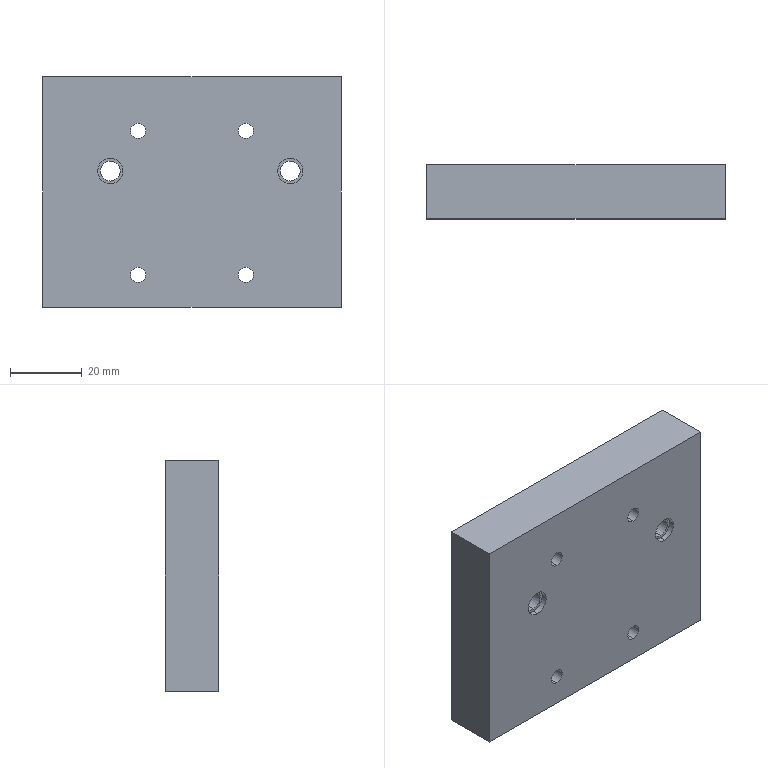Part | SolidWorks | features HoleWzd 2, ICE 2, Extrusion 1 | 1 solid | 36 faces | box 83 x 15 x 64 mm | volume 77222 mm3 | cylinder 24 | plane 12 | commonest cylinder face diameters 4.2 x8 5.5 x4 7 x4 9 x4 10 x4
STEP:
#1=CARTESIAN_POINT('',(56.5,12.9,44.5));
#2=VERTEX_POINT('',#1);
#3=CARTESIAN_POINT('',(56.5,12.9,53.5));
#4=VERTEX_POINT('',#3);
#5=CARTESIAN_POINT('',(56.5,12.9,49.));
#6=DIRECTION('',(0.,1.,0.));
#7=DIRECTION('',(0.,0.,1.));
#8=AXIS2_PLACEMENT_3D('',#5,#6,#7);
#9=CIRCLE('',#8,4.5);
#10=EDGE_CURVE('',#2,#4,#9,.T.);
#11=ORIENTED_EDGE('',*,*,#10,.F.);
#12=CARTESIAN_POINT('',(56.5,15.,44.5));
#13=VERTEX_POINT('',#12);
#14=CARTESIAN_POINT('',(56.5,12.9,44.5));
#15=DIRECTION('',(0.,1.,0.));
#16=VECTOR('',#15,1000.);
#17=LINE('',#14,#16);
#18=EDGE_CURVE('',#2,#13,#17,.T.);
#19=ORIENTED_EDGE('',*,*,#18,.T.);
#20=CARTESIAN_POINT('',(56.5,15.,53.5));
#21=VERTEX_POINT('',#20);
#22=CARTESIAN_POINT('',(56.5,15.,49.));
#23=DIRECTION('',(0.,1.,0.));
#24=DIRECTION('',(0.,0.,1.));
#25=AXIS2_PLACEMENT_3D('',#22,#23,#24);
#26=CIRCLE('',#25,4.5);
#27=EDGE_CURVE('',#13,#21,#26,.T.);
#28=ORIENTED_EDGE('',*,*,#27,.T.);
#29=CARTESIAN_POINT('',(56.5,12.9,53.5));
#30=DIRECTION('',(0.,1.,0.));
#31=VECTOR('',#30,1000.);
#32=LINE('',#29,#31);
#33=EDGE_CURVE('',#4,#21,#32,.T.);
#34=ORIENTED_EDGE('',*,*,#33,.F.);
#35=EDGE_LOOP('',(#11,#19,#28,#34));
#36=FACE_OUTER_BOUND('',#35,.T.);
#37=CARTESIAN_POINT('',(56.5,12.9,49.));
#38=DIRECTION('',(0.,1.,0.));
#39=DIRECTION('',(0.,0.,1.));
#40=AXIS2_PLACEMENT_3D('',#37,#38,#39);
#41=CYLINDRICAL_SURFACE('',#40,4.5);
#42=ADVANCED_FACE('',(#36),#41,.F.);
#43=CARTESIAN_POINT('',(26.5,12.9,44.5));
#44=VERTEX_POINT('',#43);
#45=CARTESIAN_POINT('',(26.5,12.9,53.5));
#46=VERTEX_POINT('',#45);
#47=CARTESIAN_POINT('',(26.5,12.9,49.));
#48=DIRECTION('',(0.,1.,0.));
#49=DIRECTION('',(0.,0.,1.));
#50=AXIS2_PLACEMENT_3D('',#47,#48,#49);
#51=CIRCLE('',#50,4.5);
#52=EDGE_CURVE('',#44,#46,#51,.T.);
#53=ORIENTED_EDGE('',*,*,#52,.F.);
#54=CARTESIAN_POINT('',(26.5,15.,44.5));
#55=VERTEX_POINT('',#54);
#56=CARTESIAN_POINT('',(26.5,12.9,44.5));
#57=DIRECTION('',(0.,1.,0.));
#58=VECTOR('',#57,1000.);
#59=LINE('',#56,#58);
#60=EDGE_CURVE('',#44,#55,#59,.T.);
#61=ORIENTED_EDGE('',*,*,#60,.T.);
#62=CARTESIAN_POINT('',(26.5,15.,53.5));
#63=VERTEX_POINT('',#62);
#64=CARTESIAN_POINT('',(26.5,15.,49.));
#65=DIRECTION('',(0.,1.,0.));
#66=DIRECTION('',(0.,0.,1.));
#67=AXIS2_PLACEMENT_3D('',#64,#65,#66);
#68=CIRCLE('',#67,4.5);
#69=EDGE_CURVE('',#55,#63,#68,.T.);
#70=ORIENTED_EDGE('',*,*,#69,.T.);
#71=CARTESIAN_POINT('',(26.5,12.9,53.5));
#72=DIRECTION('',(0.,1.,0.));
#73=VECTOR('',#72,1000.);
#74=LINE('',#71,#73);
#75=EDGE_CURVE('',#46,#63,#74,.T.);
#76=ORIENTED_EDGE('',*,*,#75,.F.);
#77=EDGE_LOOP('',(#53,#61,#70,#76));
#78=FACE_OUTER_BOUND('',#77,.T.);
#79=CARTESIAN_POINT('',(26.5,12.9,49.));
#80=DIRECTION('',(0.,1.,0.));
#81=DIRECTION('',(0.,0.,1.));
#82=AXIS2_PLACEMENT_3D('',#79,#80,#81);
#83=CYLINDRICAL_SURFACE('',#82,4.5);
#84=ADVANCED_FACE('',(#78),#83,.F.);
#85=CARTESIAN_POINT('',(56.5,0.,6.9));
#86=VERTEX_POINT('',#85);
#87=CARTESIAN_POINT('',(56.5,0.,11.1));
#88=VERTEX_POINT('',#87);
#89=CARTESIAN_POINT('',(56.5,0.,9.));
#90=DIRECTION('',(0.,1.,0.));
#91=DIRECTION('',(0.,0.,1.));
#92=AXIS2_PLACEMENT_3D('',#89,#90,#91);
#93=CIRCLE('',#92,2.1);
#94=EDGE_CURVE('',#86,#88,#93,.T.);
#95=ORIENTED_EDGE('',*,*,#94,.F.);
#96=CARTESIAN_POINT('',(56.5,15.,6.9));
#97=VERTEX_POINT('',#96);
#98=CARTESIAN_POINT('',(56.5,15.,6.9));
#99=DIRECTION('',(0.,1.,0.));
#100=VECTOR('',#99,1000.);
#101=LINE('',#98,#100);
#102=EDGE_CURVE('',#86,#97,#101,.T.);
#103=ORIENTED_EDGE('',*,*,#102,.T.);
#104=CARTESIAN_POINT('',(56.5,15.,11.1));
#105=VERTEX_POINT('',#104);
#106=CARTESIAN_POINT('',(56.5,15.,9.));
#107=DIRECTION('',(0.,1.,0.));
#108=DIRECTION('',(0.,0.,1.));
#109=AXIS2_PLACEMENT_3D('',#106,#107,#108);
#110=CIRCLE('',#109,2.1);
#111=EDGE_CURVE('',#97,#105,#110,.T.);
#112=ORIENTED_EDGE('',*,*,#111,.T.);
#113=CARTESIAN_POINT('',(56.5,15.,11.1));
#114=DIRECTION('',(0.,1.,0.));
#115=VECTOR('',#114,1000.);
#116=LINE('',#113,#115);
#117=EDGE_CURVE('',#88,#105,#116,.T.);
#118=ORIENTED_EDGE('',*,*,#117,.F.);
#119=EDGE_LOOP('',(#95,#103,#112,#118));
#120=FACE_OUTER_BOUND('',#119,.T.);
#121=CARTESIAN_POINT('',(56.5,15.,9.));
#122=DIRECTION('',(0.,1.,0.));
#123=DIRECTION('',(0.,0.,1.));
#124=AXIS2_PLACEMENT_3D('',#121,#122,#123);
#125=CYLINDRICAL_SURFACE('',#124,2.1);
#126=ADVANCED_FACE('',(#120),#125,.F.);
#127=CARTESIAN_POINT('',(26.5,0.,6.9));
#128=VERTEX_POINT('',#127);
#129=CARTESIAN_POINT('',(26.5,0.,11.1));
#130=VERTEX_POINT('',#129);
#131=CARTESIAN_POINT('',(26.5,0.,9.));
#132=DIRECTION('',(0.,1.,0.));
#133=DIRECTION('',(0.,0.,1.));
#134=AXIS2_PLACEMENT_3D('',#131,#132,#133);
#135=CIRCLE('',#134,2.1);
#136=EDGE_CURVE('',#128,#130,#135,.T.);
#137=ORIENTED_EDGE('',*,*,#136,.F.);
#138=CARTESIAN_POINT('',(26.5,15.,6.9));
#139=VERTEX_POINT('',#138);
#140=CARTESIAN_POINT('',(26.5,15.,6.9));
#141=DIRECTION('',(0.,1.,0.));
#142=VECTOR('',#141,1000.);
#143=LINE('',#140,#142);
#144=EDGE_CURVE('',#128,#139,#143,.T.);
#145=ORIENTED_EDGE('',*,*,#144,.T.);
#146=CARTESIAN_POINT('',(26.5,15.,11.1));
#147=VERTEX_POINT('',#146);
#148=CARTESIAN_POINT('',(26.5,15.,9.));
#149=DIRECTION('',(0.,1.,0.));
#150=DIRECTION('',(0.,0.,1.));
#151=AXIS2_PLACEMENT_3D('',#148,#149,#150);
#152=CIRCLE('',#151,2.1);
#153=EDGE_CURVE('',#139,#147,#152,.T.);
#154=ORIENTED_EDGE('',*,*,#153,.T.);
#155=CARTESIAN_POINT('',(26.5,15.,11.1));
#156=DIRECTION('',(0.,1.,0.));
#157=VECTOR('',#156,1000.);
#158=LINE('',#155,#157);
#159=EDGE_CURVE('',#130,#147,#158,.T.);
#160=ORIENTED_EDGE('',*,*,#159,.F.);
#161=EDGE_LOOP('',(#137,#145,#154,#160));
#162=FACE_OUTER_BOUND('',#161,.T.);
#163=CARTESIAN_POINT('',(26.5,15.,9.));
#164=DIRECTION('',(0.,1.,0.));
#165=DIRECTION('',(0.,0.,1.));
#166=AXIS2_PLACEMENT_3D('',#163,#164,#165);
#167=CYLINDRICAL_SURFACE('',#166,2.1);
#168=ADVANCED_FACE('',(#162),#167,.F.);
#169=CARTESIAN_POINT('',(68.8,1.6,41.3));
#170=VERTEX_POINT('',#169);
#171=CARTESIAN_POINT('',(68.8,1.6,34.3));
#172=VERTEX_POINT('',#171);
#173=CARTESIAN_POINT('',(68.8,1.6,37.8));
#174=DIRECTION('',(0.,-1.,0.));
#175=DIRECTION('',(0.,0.,-1.));
#176=AXIS2_PLACEMENT_3D('',#173,#174,#175);
#177=CIRCLE('',#176,3.5);
#178=EDGE_CURVE('',#170,#172,#177,.T.);
#179=ORIENTED_EDGE('',*,*,#178,.F.);
#180=CARTESIAN_POINT('',(68.8,0.,41.3));
#181=VERTEX_POINT('',#180);
#182=CARTESIAN_POINT('',(68.8,1.6,41.3));
#183=DIRECTION('',(0.,-1.,0.));
#184=VECTOR('',#183,1000.);
#185=LINE('',#182,#184);
#186=EDGE_CURVE('',#170,#181,#185,.T.);
#187=ORIENTED_EDGE('',*,*,#186,.T.);
#188=CARTESIAN_POINT('',(68.8,0.,34.3));
#189=VERTEX_POINT('',#188);
#190=CARTESIAN_POINT('',(68.8,0.,37.8));
#191=DIRECTION('',(0.,-1.,0.));
#192=DIRECTION('',(0.,0.,-1.));
#193=AXIS2_PLACEMENT_3D('',#190,#191,#192);
#194=CIRCLE('',#193,3.5);
#195=EDGE_CURVE('',#181,#189,#194,.T.);
#196=ORIENTED_EDGE('',*,*,#195,.T.);
#197=CARTESIAN_POINT('',(68.8,1.6,34.3));
#198=DIRECTION('',(0.,-1.,0.));
#199=VECTOR('',#198,1000.);
#200=LINE('',#197,#199);
#201=EDGE_CURVE('',#172,#189,#200,.T.);
#202=ORIENTED_EDGE('',*,*,#201,.F.);
#203=EDGE_LOOP('',(#179,#187,#196,#202));
#204=FACE_OUTER_BOUND('',#203,.T.);
#205=CARTESIAN_POINT('',(68.8,1.6,37.8));
#206=DIRECTION('',(0.,-1.,0.));
#207=DIRECTION('',(0.,0.,-1.));
#208=AXIS2_PLACEMENT_3D('',#205,#206,#207);
#209=CYLINDRICAL_SURFACE('',#208,3.5);
#210=ADVANCED_FACE('',(#204),#209,.F.);
#211=CARTESIAN_POINT('',(18.8,1.6,41.3));
#212=VERTEX_POINT('',#211);
#213=CARTESIAN_POINT('',(18.8,1.6,34.3));
#214=VERTEX_POINT('',#213);
#215=CARTESIAN_POINT('',(18.8,1.6,37.8));
#216=DIRECTION('',(0.,-1.,0.));
#217=DIRECTION('',(0.,0.,-1.));
#218=AXIS2_PLACEMENT_3D('',#215,#216,#217);
#219=CIRCLE('',#218,3.5);
#220=EDGE_CURVE('',#212,#214,#219,.T.);
#221=ORIENTED_EDGE('',*,*,#220,.F.);
#222=CARTESIAN_POINT('',(18.8,0.,41.3));
#223=VERTEX_POINT('',#222);
#224=CARTESIAN_POINT('',(18.8,1.6,41.3));
#225=DIRECTION('',(0.,-1.,0.));
#226=VECTOR('',#225,1000.);
#227=LINE('',#224,#226);
#228=EDGE_CURVE('',#212,#223,#227,.T.);
#229=ORIENTED_EDGE('',*,*,#228,.T.);
#230=CARTESIAN_POINT('',(18.8,0.,34.3));
#231=VERTEX_POINT('',#230);
#232=CARTESIAN_POINT('',(18.8,0.,37.8));
#233=DIRECTION('',(0.,-1.,0.));
#234=DIRECTION('',(0.,0.,-1.));
#235=AXIS2_PLACEMENT_3D('',#232,#233,#234);
#236=CIRCLE('',#235,3.5);
#237=EDGE_CURVE('',#223,#231,#236,.T.);
#238=ORIENTED_EDGE('',*,*,#237,.T.);
#239=CARTESIAN_POINT('',(18.8,1.6,34.3));
#240=DIRECTION('',(0.,-1.,0.));
#241=VECTOR('',#240,1000.);
#242=LINE('',#239,#241);
#243=EDGE_CURVE('',#214,#231,#242,.T.);
#244=ORIENTED_EDGE('',*,*,#243,.F.);
#245=EDGE_LOOP('',(#221,#229,#238,#244));
#246=FACE_OUTER_BOUND('',#245,.T.);
#247=CARTESIAN_POINT('',(18.8,1.6,37.8));
#248=DIRECTION('',(0.,-1.,0.));
#249=DIRECTION('',(0.,0.,-1.));
#250=AXIS2_PLACEMENT_3D('',#247,#248,#249);
#251=CYLINDRICAL_SURFACE('',#250,3.5);
#252=ADVANCED_FACE('',(#246),#251,.F.);
#253=CARTESIAN_POINT('',(18.8,9.,32.8));
#254=VERTEX_POINT('',#253);
#255=CARTESIAN_POINT('',(18.8,9.,42.8));
#256=VERTEX_POINT('',#255);
#257=CARTESIAN_POINT('',(18.8,9.,37.8));
#258=DIRECTION('',(0.,1.,0.));
#259=DIRECTION('',(0.,0.,1.));
#260=AXIS2_PLACEMENT_3D('',#257,#258,#259);
#261=CIRCLE('',#260,5.);
#262=EDGE_CURVE('',#254,#256,#261,.T.);
#263=ORIENTED_EDGE('',*,*,#262,.F.);
#264=CARTESIAN_POINT('',(18.8,15.,32.8));
#265=VERTEX_POINT('',#264);
#266=CARTESIAN_POINT('',(18.8,15.,32.8));
#267=DIRECTION('',(0.,1.,0.));
#268=VECTOR('',#267,1000.);
#269=LINE('',#266,#268);
#270=EDGE_CURVE('',#254,#265,#269,.T.);
#271=ORIENTED_EDGE('',*,*,#270,.T.);
#272=CARTESIAN_POINT('',(18.8,15.,42.8));
#273=VERTEX_POINT('',#272);
#274=CARTESIAN_POINT('',(18.8,15.,37.8));
#275=DIRECTION('',(0.,1.,0.));
#276=DIRECTION('',(0.,0.,1.));
#277=AXIS2_PLACEMENT_3D('',#274,#275,#276);
#278=CIRCLE('',#277,5.);
#279=EDGE_CURVE('',#265,#273,#278,.T.);
#280=ORIENTED_EDGE('',*,*,#279,.T.);
#281=CARTESIAN_POINT('',(18.8,15.,42.8));
#282=DIRECTION('',(0.,1.,0.));
#283=VECTOR('',#282,1000.);
#284=LINE('',#281,#283);
#285=EDGE_CURVE('',#256,#273,#284,.T.);
#286=ORIENTED_EDGE('',*,*,#285,.F.);
#287=EDGE_LOOP('',(#263,#271,#280,#286));
#288=FACE_OUTER_BOUND('',#287,.T.);
#289=CARTESIAN_POINT('',(18.8,15.,37.8));
#290=DIRECTION('',(0.,1.,0.));
#291=DIRECTION('',(0.,0.,1.));
#292=AXIS2_PLACEMENT_3D('',#289,#290,#291);
#293=CYLINDRICAL_SURFACE('',#292,5.);
#294=ADVANCED_FACE('',(#288),#293,.F.);
#295=CARTESIAN_POINT('',(68.8,9.,32.8));
#296=VERTEX_POINT('',#295);
#297=CARTESIAN_POINT('',(68.8,9.,42.8));
#298=VERTEX_POINT('',#297);
#299=CARTESIAN_POINT('',(68.8,9.,37.8));
#300=DIRECTION('',(0.,1.,0.));
#301=DIRECTION('',(0.,0.,1.));
#302=AXIS2_PLACEMENT_3D('',#299,#300,#301);
#303=CIRCLE('',#302,5.);
#304=EDGE_CURVE('',#296,#298,#303,.T.);
#305=ORIENTED_EDGE('',*,*,#304,.F.);
#306=CARTESIAN_POINT('',(68.8,15.,32.8));
#307=VERTEX_POINT('',#306);
#308=CARTESIAN_POINT('',(68.8,15.,32.8));
#309=DIRECTION('',(0.,1.,0.));
#310=VECTOR('',#309,1000.);
#311=LINE('',#308,#310);
#312=EDGE_CURVE('',#296,#307,#311,.T.);
#313=ORIENTED_EDGE('',*,*,#312,.T.);
#314=CARTESIAN_POINT('',(68.8,15.,42.8));
#315=VERTEX_POINT('',#314);
#316=CARTESIAN_POINT('',(68.8,15.,37.8));
#317=DIRECTION('',(0.,1.,0.));
#318=DIRECTION('',(0.,0.,1.));
#319=AXIS2_PLACEMENT_3D('',#316,#317,#318);
#320=CIRCLE('',#319,5.);
#321=EDGE_CURVE('',#307,#315,#320,.T.);
#322=ORIENTED_EDGE('',*,*,#321,.T.);
#323=CARTESIAN_POINT('',(68.8,15.,42.8));
#324=DIRECTION('',(0.,1.,0.));
#325=VECTOR('',#324,1000.);
#326=LINE('',#323,#325);
#327=EDGE_CURVE('',#298,#315,#326,.T.);
#328=ORIENTED_EDGE('',*,*,#327,.F.);
#329=EDGE_LOOP('',(#305,#313,#322,#328));
#330=FACE_OUTER_BOUND('',#329,.T.);
#331=CARTESIAN_POINT('',(68.8,15.,37.8));
#332=DIRECTION('',(0.,1.,0.));
#333=DIRECTION('',(0.,0.,1.));
#334=AXIS2_PLACEMENT_3D('',#331,#332,#333);
#335=CYLINDRICAL_SURFACE('',#334,5.);
#336=ADVANCED_FACE('',(#330),#335,.F.);
#337=CARTESIAN_POINT('',(18.8,1.6,35.05));
#338=VERTEX_POINT('',#337);
#339=CARTESIAN_POINT('',(18.8,1.6,40.55));
#340=VERTEX_POINT('',#339);
#341=CARTESIAN_POINT('',(18.8,1.6,37.8));
#342=DIRECTION('',(0.,1.,0.));
#343=DIRECTION('',(0.,0.,-1.));
#344=AXIS2_PLACEMENT_3D('',#341,#342,#343);
#345=CIRCLE('',#344,2.75);
#346=EDGE_CURVE('',#338,#340,#345,.T.);
#347=ORIENTED_EDGE('',*,*,#346,.F.);
#348=CARTESIAN_POINT('',(18.8,9.,35.05));
#349=VERTEX_POINT('',#348);
#350=CARTESIAN_POINT('',(18.8,15.,35.05));
#351=DIRECTION('',(0.,1.,0.));
#352=VECTOR('',#351,1000.);
#353=LINE('',#350,#352);
#354=EDGE_CURVE('',#338,#349,#353,.T.);
#355=ORIENTED_EDGE('',*,*,#354,.T.);
#356=CARTESIAN_POINT('',(18.8,9.,40.55));
#357=VERTEX_POINT('',#356);
#358=CARTESIAN_POINT('',(18.8,9.,37.8));
#359=DIRECTION('',(0.,1.,0.));
#360=DIRECTION('',(0.,0.,1.));
#361=AXIS2_PLACEMENT_3D('',#358,#359,#360);
#362=CIRCLE('',#361,2.75);
#363=EDGE_CURVE('',#349,#357,#362,.T.);
#364=ORIENTED_EDGE('',*,*,#363,.T.);
#365=CARTESIAN_POINT('',(18.8,15.,40.55));
#366=DIRECTION('',(0.,1.,0.));
#367=VECTOR('',#366,1000.);
#368=LINE('',#365,#367);
#369=EDGE_CURVE('',#340,#357,#368,.T.);
#370=ORIENTED_EDGE('',*,*,#369,.F.);
#371=EDGE_LOOP('',(#347,#355,#364,#370));
#372=FACE_OUTER_BOUND('',#371,.T.);
#373=CARTESIAN_POINT('',(18.8,15.,37.8));
#374=DIRECTION('',(0.,1.,0.));
#375=DIRECTION('',(0.,0.,1.));
#376=AXIS2_PLACEMENT_3D('',#373,#374,#375);
#377=CYLINDRICAL_SURFACE('',#376,2.75);
#378=ADVANCED_FACE('',(#372),#377,.F.);
#379=CARTESIAN_POINT('',(68.8,1.6,35.05));
#380=VERTEX_POINT('',#379);
#381=CARTESIAN_POINT('',(68.8,1.6,40.55));
#382=VERTEX_POINT('',#381);
#383=CARTESIAN_POINT('',(68.8,1.6,37.8));
#384=DIRECTION('',(0.,1.,0.));
#385=DIRECTION('',(0.,0.,-1.));
#386=AXIS2_PLACEMENT_3D('',#383,#384,#385);
#387=CIRCLE('',#386,2.75);
#388=EDGE_CURVE('',#380,#382,#387,.T.);
#389=ORIENTED_EDGE('',*,*,#388,.F.);
#390=CARTESIAN_POINT('',(68.8,9.,35.05));
#391=VERTEX_POINT('',#390);
#392=CARTESIAN_POINT('',(68.8,15.,35.05));
#393=DIRECTION('',(0.,1.,0.));
#394=VECTOR('',#393,1000.);
#395=LINE('',#392,#394);
#396=EDGE_CURVE('',#380,#391,#395,.T.);
#397=ORIENTED_EDGE('',*,*,#396,.T.);
#398=CARTESIAN_POINT('',(68.8,9.,40.55));
#399=VERTEX_POINT('',#398);
#400=CARTESIAN_POINT('',(68.8,9.,37.8));
#401=DIRECTION('',(0.,1.,0.));
#402=DIRECTION('',(0.,0.,1.));
#403=AXIS2_PLACEMENT_3D('',#400,#401,#402);
#404=CIRCLE('',#403,2.75);
#405=EDGE_CURVE('',#391,#399,#404,.T.);
#406=ORIENTED_EDGE('',*,*,#405,.T.);
#407=CARTESIAN_POINT('',(68.8,15.,40.55));
#408=DIRECTION('',(0.,1.,0.));
#409=VECTOR('',#408,1000.);
#410=LINE('',#407,#409);
#411=EDGE_CURVE('',#382,#399,#410,.T.);
#412=ORIENTED_EDGE('',*,*,#411,.F.);
#413=EDGE_LOOP('',(#389,#397,#406,#412));
#414=FACE_OUTER_BOUND('',#413,.T.);
#415=CARTESIAN_POINT('',(68.8,15.,37.8));
#416=DIRECTION('',(0.,1.,0.));
#417=DIRECTION('',(0.,0.,1.));
#418=AXIS2_PLACEMENT_3D('',#415,#416,#417);
#419=CYLINDRICAL_SURFACE('',#418,2.75);
#420=ADVANCED_FACE('',(#414),#419,.F.);
#421=CARTESIAN_POINT('',(26.5,0.,46.9));
#422=VERTEX_POINT('',#421);
#423=CARTESIAN_POINT('',(26.5,0.,51.1));
#424=VERTEX_POINT('',#423);
#425=CARTESIAN_POINT('',(26.5,0.,49.));
#426=DIRECTION('',(0.,1.,0.));
#427=DIRECTION('',(0.,0.,1.));
#428=AXIS2_PLACEMENT_3D('',#425,#426,#427);
#429=CIRCLE('',#428,2.1);
#430=EDGE_CURVE('',#422,#424,#429,.T.);
#431=ORIENTED_EDGE('',*,*,#430,.F.);
#432=CARTESIAN_POINT('',(26.5,12.9,46.9));
#433=VERTEX_POINT('',#432);
#434=CARTESIAN_POINT('',(26.5,15.,46.9));
#435=DIRECTION('',(0.,1.,0.));
#436=VECTOR('',#435,1000.);
#437=LINE('',#434,#436);
#438=EDGE_CURVE('',#422,#433,#437,.T.);
#439=ORIENTED_EDGE('',*,*,#438,.T.);
#440=CARTESIAN_POINT('',(26.5,12.9,51.1));
#441=VERTEX_POINT('',#440);
#442=CARTESIAN_POINT('',(26.5,12.9,49.));
#443=DIRECTION('',(0.,-1.,0.));
#444=DIRECTION('',(0.,0.,1.));
#445=AXIS2_PLACEMENT_3D('',#442,#443,#444);
#446=CIRCLE('',#445,2.1);
#447=EDGE_CURVE('',#441,#433,#446,.T.);
#448=ORIENTED_EDGE('',*,*,#447,.F.);
#449=CARTESIAN_POINT('',(26.5,15.,51.1));
#450=DIRECTION('',(0.,1.,0.));
#451=VECTOR('',#450,1000.);
#452=LINE('',#449,#451);
#453=EDGE_CURVE('',#424,#441,#452,.T.);
#454=ORIENTED_EDGE('',*,*,#453,.F.);
#455=EDGE_LOOP('',(#431,#439,#448,#454));
#456=FACE_OUTER_BOUND('',#455,.T.);
#457=CARTESIAN_POINT('',(26.5,15.,49.));
#458=DIRECTION('',(0.,1.,0.));
#459=DIRECTION('',(0.,0.,1.));
#460=AXIS2_PLACEMENT_3D('',#457,#458,#459);
#461=CYLINDRICAL_SURFACE('',#460,2.1);
#462=ADVANCED_FACE('',(#456),#461,.F.);
#463=CARTESIAN_POINT('',(56.5,0.,46.9));
#464=VERTEX_POINT('',#463);
#465=CARTESIAN_POINT('',(56.5,0.,51.1));
#466=VERTEX_POINT('',#465);
#467=CARTESIAN_POINT('',(56.5,0.,49.));
#468=DIRECTION('',(0.,1.,0.));
#469=DIRECTION('',(0.,0.,1.));
#470=AXIS2_PLACEMENT_3D('',#467,#468,#469);
#471=CIRCLE('',#470,2.1);
#472=EDGE_CURVE('',#464,#466,#471,.T.);
#473=ORIENTED_EDGE('',*,*,#472,.F.);
#474=CARTESIAN_POINT('',(56.5,12.9,46.9));
#475=VERTEX_POINT('',#474);
#476=CARTESIAN_POINT('',(56.5,15.,46.9));
#477=DIRECTION('',(0.,1.,0.));
#478=VECTOR('',#477,1000.);
#479=LINE('',#476,#478);
#480=EDGE_CURVE('',#464,#475,#479,.T.);
#481=ORIENTED_EDGE('',*,*,#480,.T.);
#482=CARTESIAN_POINT('',(56.5,12.9,51.1));
#483=VERTEX_POINT('',#482);
#484=CARTESIAN_POINT('',(56.5,12.9,49.));
#485=DIRECTION('',(0.,-1.,0.));
#486=DIRECTION('',(0.,0.,1.));
#487=AXIS2_PLACEMENT_3D('',#484,#485,#486);
#488=CIRCLE('',#487,2.1);
#489=EDGE_CURVE('',#483,#475,#488,.T.);
#490=ORIENTED_EDGE('',*,*,#489,.F.);
#491=CARTESIAN_POINT('',(56.5,15.,51.1));
#492=DIRECTION('',(0.,1.,0.));
#493=VECTOR('',#492,1000.);
#494=LINE('',#491,#493);
#495=EDGE_CURVE('',#466,#483,#494,.T.);
#496=ORIENTED_EDGE('',*,*,#495,.F.);
#497=EDGE_LOOP('',(#473,#481,#490,#496));
#498=FACE_OUTER_BOUND('',#497,.T.);
#499=CARTESIAN_POINT('',(56.5,15.,49.));
#500=DIRECTION('',(0.,1.,0.));
#501=DIRECTION('',(0.,0.,1.));
#502=AXIS2_PLACEMENT_3D('',#499,#500,#501);
#503=CYLINDRICAL_SURFACE('',#502,2.1);
#504=ADVANCED_FACE('',(#498),#503,.F.);
#505=ORIENTED_EDGE('',*,*,#480,.F.);
#506=CARTESIAN_POINT('',(56.5,0.,49.));
#507=DIRECTION('',(0.,1.,0.));
#508=DIRECTION('',(0.,0.,1.));
#509=AXIS2_PLACEMENT_3D('',#506,#507,#508);
#510=CIRCLE('',#509,2.1);
#511=EDGE_CURVE('',#466,#464,#510,.T.);
#512=ORIENTED_EDGE('',*,*,#511,.F.);
#513=ORIENTED_EDGE('',*,*,#495,.T.);
#514=CARTESIAN_POINT('',(56.5,12.9,49.));
#515=DIRECTION('',(0.,-1.,0.));
#516=DIRECTION('',(0.,0.,1.));
#517=AXIS2_PLACEMENT_3D('',#514,#515,#516);
#518=CIRCLE('',#517,2.1);
#519=EDGE_CURVE('',#475,#483,#518,.T.);
#520=ORIENTED_EDGE('',*,*,#519,.F.);
#521=EDGE_LOOP('',(#505,#512,#513,#520));
#522=FACE_OUTER_BOUND('',#521,.T.);
#523=CARTESIAN_POINT('',(56.5,15.,49.));
#524=DIRECTION('',(0.,1.,0.));
#525=DIRECTION('',(0.,0.,1.));
#526=AXIS2_PLACEMENT_3D('',#523,#524,#525);
#527=CYLINDRICAL_SURFACE('',#526,2.1);
#528=ADVANCED_FACE('',(#522),#527,.F.);
#529=ORIENTED_EDGE('',*,*,#438,.F.);
#530=CARTESIAN_POINT('',(26.5,0.,49.));
#531=DIRECTION('',(0.,1.,0.));
#532=DIRECTION('',(0.,0.,1.));
#533=AXIS2_PLACEMENT_3D('',#530,#531,#532);
#534=CIRCLE('',#533,2.1);
#535=EDGE_CURVE('',#424,#422,#534,.T.);
#536=ORIENTED_EDGE('',*,*,#535,.F.);
#537=ORIENTED_EDGE('',*,*,#453,.T.);
#538=CARTESIAN_POINT('',(26.5,12.9,49.));
#539=DIRECTION('',(0.,-1.,0.));
#540=DIRECTION('',(0.,0.,1.));
#541=AXIS2_PLACEMENT_3D('',#538,#539,#540);
#542=CIRCLE('',#541,2.1);
#543=EDGE_CURVE('',#433,#441,#542,.T.);
#544=ORIENTED_EDGE('',*,*,#543,.F.);
#545=EDGE_LOOP('',(#529,#536,#537,#544));
#546=FACE_OUTER_BOUND('',#545,.T.);
#547=CARTESIAN_POINT('',(26.5,15.,49.));
#548=DIRECTION('',(0.,1.,0.));
#549=DIRECTION('',(0.,0.,1.));
#550=AXIS2_PLACEMENT_3D('',#547,#548,#549);
#551=CYLINDRICAL_SURFACE('',#550,2.1);
#552=ADVANCED_FACE('',(#546),#551,.F.);
#553=ORIENTED_EDGE('',*,*,#396,.F.);
#554=CARTESIAN_POINT('',(68.8,1.6,37.8));
#555=DIRECTION('',(0.,1.,0.));
#556=DIRECTION('',(0.,0.,-1.));
#557=AXIS2_PLACEMENT_3D('',#554,#555,#556);
#558=CIRCLE('',#557,2.75);
#559=EDGE_CURVE('',#382,#380,#558,.T.);
#560=ORIENTED_EDGE('',*,*,#559,.F.);
#561=ORIENTED_EDGE('',*,*,#411,.T.);
#562=CARTESIAN_POINT('',(68.8,9.,37.8));
#563=DIRECTION('',(0.,1.,0.));
#564=DIRECTION('',(0.,0.,1.));
#565=AXIS2_PLACEMENT_3D('',#562,#563,#564);
#566=CIRCLE('',#565,2.75);
#567=EDGE_CURVE('',#399,#391,#566,.T.);
#568=ORIENTED_EDGE('',*,*,#567,.T.);
#569=EDGE_LOOP('',(#553,#560,#561,#568));
#570=FACE_OUTER_BOUND('',#569,.T.);
#571=CARTESIAN_POINT('',(68.8,15.,37.8));
#572=DIRECTION('',(0.,1.,0.));
#573=DIRECTION('',(0.,0.,1.));
#574=AXIS2_PLACEMENT_3D('',#571,#572,#573);
#575=CYLINDRICAL_SURFACE('',#574,2.75);
#576=ADVANCED_FACE('',(#570),#575,.F.);
#577=ORIENTED_EDGE('',*,*,#354,.F.);
#578=CARTESIAN_POINT('',(18.8,1.6,37.8));
#579=DIRECTION('',(0.,1.,0.));
#580=DIRECTION('',(0.,0.,-1.));
#581=AXIS2_PLACEMENT_3D('',#578,#579,#580);
#582=CIRCLE('',#581,2.75);
#583=EDGE_CURVE('',#340,#338,#582,.T.);
#584=ORIENTED_EDGE('',*,*,#583,.F.);
#585=ORIENTED_EDGE('',*,*,#369,.T.);
#586=CARTESIAN_POINT('',(18.8,9.,37.8));
#587=DIRECTION('',(0.,1.,0.));
#588=DIRECTION('',(0.,0.,1.));
#589=AXIS2_PLACEMENT_3D('',#586,#587,#588);
#590=CIRCLE('',#589,2.75);
#591=EDGE_CURVE('',#357,#349,#590,.T.);
#592=ORIENTED_EDGE('',*,*,#591,.T.);
#593=EDGE_LOOP('',(#577,#584,#585,#592));
#594=FACE_OUTER_BOUND('',#593,.T.);
#595=CARTESIAN_POINT('',(18.8,15.,37.8));
#596=DIRECTION('',(0.,1.,0.));
#597=DIRECTION('',(0.,0.,1.));
#598=AXIS2_PLACEMENT_3D('',#595,#596,#597);
#599=CYLINDRICAL_SURFACE('',#598,2.75);
#600=ADVANCED_FACE('',(#594),#599,.F.);
#601=CARTESIAN_POINT('',(0.,15.,0.));
#602=VERTEX_POINT('',#601);
#603=CARTESIAN_POINT('',(0.,0.,0.));
#604=VERTEX_POINT('',#603);
#605=CARTESIAN_POINT('',(0.,0.,0.));
#606=DIRECTION('',(0.,-1.,0.));
#607=VECTOR('',#606,1000.);
#608=LINE('',#605,#607);
#609=EDGE_CURVE('',#602,#604,#608,.T.);
#610=ORIENTED_EDGE('',*,*,#609,.T.);
#611=CARTESIAN_POINT('',(0.,0.,64.));
#612=VERTEX_POINT('',#611);
#613=CARTESIAN_POINT('',(0.,0.,64.));
#614=DIRECTION('',(0.,0.,-1.));
#615=VECTOR('',#614,1000.);
#616=LINE('',#613,#615);
#617=EDGE_CURVE('',#612,#604,#616,.T.);
#618=ORIENTED_EDGE('',*,*,#617,.F.);
#619=CARTESIAN_POINT('',(0.,15.,64.));
#620=VERTEX_POINT('',#619);
#621=CARTESIAN_POINT('',(0.,0.,64.));
#622=DIRECTION('',(0.,-1.,0.));
#623=VECTOR('',#622,1000.);
#624=LINE('',#621,#623);
#625=EDGE_CURVE('',#620,#612,#624,.T.);
#626=ORIENTED_EDGE('',*,*,#625,.F.);
#627=CARTESIAN_POINT('',(0.,15.,64.));
#628=DIRECTION('',(0.,0.,-1.));
#629=VECTOR('',#628,1000.);
#630=LINE('',#627,#629);
#631=EDGE_CURVE('',#620,#602,#630,.T.);
#632=ORIENTED_EDGE('',*,*,#631,.T.);
#633=EDGE_LOOP('',(#610,#618,#626,#632));
#634=FACE_OUTER_BOUND('',#633,.T.);
#635=CARTESIAN_POINT('',(0.,0.,64.));
#636=DIRECTION('',(1.,0.,0.));
#637=DIRECTION('',(0.,0.,-1.));
#638=AXIS2_PLACEMENT_3D('',#635,#636,#637);
#639=PLANE('',#638);
#640=ADVANCED_FACE('',(#634),#639,.F.);
#641=CARTESIAN_POINT('',(56.5,0.,9.));
#642=DIRECTION('',(0.,1.,0.));
#643=DIRECTION('',(0.,0.,1.));
#644=AXIS2_PLACEMENT_3D('',#641,#642,#643);
#645=CIRCLE('',#644,2.1);
#646=EDGE_CURVE('',#88,#86,#645,.T.);
#647=ORIENTED_EDGE('',*,*,#646,.T.);
#648=ORIENTED_EDGE('',*,*,#94,.T.);
#649=EDGE_LOOP('',(#647,#648));
#650=FACE_BOUND('',#649,.T.);
#651=CARTESIAN_POINT('',(26.5,0.,9.));
#652=DIRECTION('',(0.,1.,0.));
#653=DIRECTION('',(0.,0.,1.));
#654=AXIS2_PLACEMENT_3D('',#651,#652,#653);
#655=CIRCLE('',#654,2.1);
#656=EDGE_CURVE('',#130,#128,#655,.T.);
#657=ORIENTED_EDGE('',*,*,#656,.T.);
#658=ORIENTED_EDGE('',*,*,#136,.T.);
#659=EDGE_LOOP('',(#657,#658));
#660=FACE_BOUND('',#659,.T.);
#661=ORIENTED_EDGE('',*,*,#535,.T.);
#662=ORIENTED_EDGE('',*,*,#430,.T.);
#663=EDGE_LOOP('',(#661,#662));
#664=FACE_BOUND('',#663,.T.);
#665=ORIENTED_EDGE('',*,*,#511,.T.);
#666=ORIENTED_EDGE('',*,*,#472,.T.);
#667=EDGE_LOOP('',(#665,#666));
#668=FACE_BOUND('',#667,.T.);
#669=CARTESIAN_POINT('',(68.8,0.,37.8));
#670=DIRECTION('',(0.,-1.,0.));
#671=DIRECTION('',(0.,0.,-1.));
#672=AXIS2_PLACEMENT_3D('',#669,#670,#671);
#673=CIRCLE('',#672,3.5);
#674=EDGE_CURVE('',#189,#181,#673,.T.);
#675=ORIENTED_EDGE('',*,*,#674,.F.);
#676=ORIENTED_EDGE('',*,*,#195,.F.);
#677=EDGE_LOOP('',(#675,#676));
#678=FACE_BOUND('',#677,.T.);
#679=CARTESIAN_POINT('',(18.8,0.,37.8));
#680=DIRECTION('',(0.,-1.,0.));
#681=DIRECTION('',(0.,0.,-1.));
#682=AXIS2_PLACEMENT_3D('',#679,#680,#681);
#683=CIRCLE('',#682,3.5);
#684=EDGE_CURVE('',#231,#223,#683,.T.);
#685=ORIENTED_EDGE('',*,*,#684,.F.);
#686=ORIENTED_EDGE('',*,*,#237,.F.);
#687=EDGE_LOOP('',(#685,#686));
#688=FACE_BOUND('',#687,.T.);
#689=CARTESIAN_POINT('',(83.,0.,0.));
#690=VERTEX_POINT('',#689);
#691=CARTESIAN_POINT('',(0.,0.,0.));
#692=DIRECTION('',(1.,0.,0.));
#693=VECTOR('',#692,1000.);
#694=LINE('',#691,#693);
#695=EDGE_CURVE('',#604,#690,#694,.T.);
#696=ORIENTED_EDGE('',*,*,#695,.T.);
#697=CARTESIAN_POINT('',(83.,0.,64.));
#698=VERTEX_POINT('',#697);
#699=CARTESIAN_POINT('',(83.,0.,64.));
#700=DIRECTION('',(0.,0.,-1.));
#701=VECTOR('',#700,1000.);
#702=LINE('',#699,#701);
#703=EDGE_CURVE('',#698,#690,#702,.T.);
#704=ORIENTED_EDGE('',*,*,#703,.F.);
#705=CARTESIAN_POINT('',(0.,0.,64.));
#706=DIRECTION('',(1.,0.,0.));
#707=VECTOR('',#706,1000.);
#708=LINE('',#705,#707);
#709=EDGE_CURVE('',#612,#698,#708,.T.);
#710=ORIENTED_EDGE('',*,*,#709,.F.);
#711=ORIENTED_EDGE('',*,*,#617,.T.);
#712=EDGE_LOOP('',(#696,#704,#710,#711));
#713=FACE_OUTER_BOUND('',#712,.T.);
#714=CARTESIAN_POINT('',(0.,0.,64.));
#715=DIRECTION('',(0.,1.,0.));
#716=DIRECTION('',(0.,0.,1.));
#717=AXIS2_PLACEMENT_3D('',#714,#715,#716);
#718=PLANE('',#717);
#719=ADVANCED_FACE('',(#650,#660,#664,#668,#678,#688,#713),#718,.F.);
#720=CARTESIAN_POINT('',(83.,15.,0.));
#721=VERTEX_POINT('',#720);
#722=CARTESIAN_POINT('',(83.,0.,0.));
#723=DIRECTION('',(0.,1.,0.));
#724=VECTOR('',#723,1000.);
#725=LINE('',#722,#724);
#726=EDGE_CURVE('',#690,#721,#725,.T.);
#727=ORIENTED_EDGE('',*,*,#726,.T.);
#728=CARTESIAN_POINT('',(83.,15.,64.));
#729=VERTEX_POINT('',#728);
#730=CARTESIAN_POINT('',(83.,15.,64.));
#731=DIRECTION('',(0.,0.,-1.));
#732=VECTOR('',#731,1000.);
#733=LINE('',#730,#732);
#734=EDGE_CURVE('',#729,#721,#733,.T.);
#735=ORIENTED_EDGE('',*,*,#734,.F.);
#736=CARTESIAN_POINT('',(83.,0.,64.));
#737=DIRECTION('',(0.,1.,0.));
#738=VECTOR('',#737,1000.);
#739=LINE('',#736,#738);
#740=EDGE_CURVE('',#698,#729,#739,.T.);
#741=ORIENTED_EDGE('',*,*,#740,.F.);
#742=ORIENTED_EDGE('',*,*,#703,.T.);
#743=EDGE_LOOP('',(#727,#735,#741,#742));
#744=FACE_OUTER_BOUND('',#743,.T.);
#745=CARTESIAN_POINT('',(83.,0.,64.));
#746=DIRECTION('',(-1.,0.,0.));
#747=DIRECTION('',(0.,0.,1.));
#748=AXIS2_PLACEMENT_3D('',#745,#746,#747);
#749=PLANE('',#748);
#750=ADVANCED_FACE('',(#744),#749,.F.);
#751=CARTESIAN_POINT('',(56.5,15.,49.));
#752=DIRECTION('',(0.,1.,0.));
#753=DIRECTION('',(0.,0.,1.));
#754=AXIS2_PLACEMENT_3D('',#751,#752,#753);
#755=CIRCLE('',#754,4.5);
#756=EDGE_CURVE('',#21,#13,#755,.T.);
#757=ORIENTED_EDGE('',*,*,#756,.F.);
#758=ORIENTED_EDGE('',*,*,#27,.F.);
#759=EDGE_LOOP('',(#757,#758));
#760=FACE_BOUND('',#759,.T.);
#761=CARTESIAN_POINT('',(26.5,15.,49.));
#762=DIRECTION('',(0.,1.,0.));
#763=DIRECTION('',(0.,0.,1.));
#764=AXIS2_PLACEMENT_3D('',#761,#762,#763);
#765=CIRCLE('',#764,4.5);
#766=EDGE_CURVE('',#63,#55,#765,.T.);
#767=ORIENTED_EDGE('',*,*,#766,.F.);
#768=ORIENTED_EDGE('',*,*,#69,.F.);
#769=EDGE_LOOP('',(#767,#768));
#770=FACE_BOUND('',#769,.T.);
#771=CARTESIAN_POINT('',(56.5,15.,9.));
#772=DIRECTION('',(0.,1.,0.));
#773=DIRECTION('',(0.,0.,1.));
#774=AXIS2_PLACEMENT_3D('',#771,#772,#773);
#775=CIRCLE('',#774,2.1);
#776=EDGE_CURVE('',#105,#97,#775,.T.);
#777=ORIENTED_EDGE('',*,*,#776,.F.);
#778=ORIENTED_EDGE('',*,*,#111,.F.);
#779=EDGE_LOOP('',(#777,#778));
#780=FACE_BOUND('',#779,.T.);
#781=CARTESIAN_POINT('',(26.5,15.,9.));
#782=DIRECTION('',(0.,1.,0.));
#783=DIRECTION('',(0.,0.,1.));
#784=AXIS2_PLACEMENT_3D('',#781,#782,#783);
#785=CIRCLE('',#784,2.1);
#786=EDGE_CURVE('',#147,#139,#785,.T.);
#787=ORIENTED_EDGE('',*,*,#786,.F.);
#788=ORIENTED_EDGE('',*,*,#153,.F.);
#789=EDGE_LOOP('',(#787,#788));
#790=FACE_BOUND('',#789,.T.);
#791=CARTESIAN_POINT('',(18.8,15.,37.8));
#792=DIRECTION('',(0.,1.,0.));
#793=DIRECTION('',(0.,0.,1.));
#794=AXIS2_PLACEMENT_3D('',#791,#792,#793);
#795=CIRCLE('',#794,5.);
#796=EDGE_CURVE('',#273,#265,#795,.T.);
#797=ORIENTED_EDGE('',*,*,#796,.F.);
#798=ORIENTED_EDGE('',*,*,#279,.F.);
#799=EDGE_LOOP('',(#797,#798));
#800=FACE_BOUND('',#799,.T.);
#801=CARTESIAN_POINT('',(68.8,15.,37.8));
#802=DIRECTION('',(0.,1.,0.));
#803=DIRECTION('',(0.,0.,1.));
#804=AXIS2_PLACEMENT_3D('',#801,#802,#803);
#805=CIRCLE('',#804,5.);
#806=EDGE_CURVE('',#315,#307,#805,.T.);
#807=ORIENTED_EDGE('',*,*,#806,.F.);
#808=ORIENTED_EDGE('',*,*,#321,.F.);
#809=EDGE_LOOP('',(#807,#808));
#810=FACE_BOUND('',#809,.T.);
#811=CARTESIAN_POINT('',(0.,15.,0.));
#812=DIRECTION('',(-1.,0.,0.));
#813=VECTOR('',#812,1000.);
#814=LINE('',#811,#813);
#815=EDGE_CURVE('',#721,#602,#814,.T.);
#816=ORIENTED_EDGE('',*,*,#815,.T.);
#817=ORIENTED_EDGE('',*,*,#631,.F.);
#818=CARTESIAN_POINT('',(0.,15.,64.));
#819=DIRECTION('',(-1.,0.,0.));
#820=VECTOR('',#819,1000.);
#821=LINE('',#818,#820);
#822=EDGE_CURVE('',#729,#620,#821,.T.);
#823=ORIENTED_EDGE('',*,*,#822,.F.);
#824=ORIENTED_EDGE('',*,*,#734,.T.);
#825=EDGE_LOOP('',(#816,#817,#823,#824));
#826=FACE_OUTER_BOUND('',#825,.T.);
#827=CARTESIAN_POINT('',(0.,15.,64.));
#828=DIRECTION('',(0.,-1.,0.));
#829=DIRECTION('',(0.,0.,-1.));
#830=AXIS2_PLACEMENT_3D('',#827,#828,#829);
#831=PLANE('',#830);
#832=ADVANCED_FACE('',(#760,#770,#780,#790,#800,#810,#826),#831,.F.);
#833=ORIENTED_EDGE('',*,*,#625,.T.);
#834=ORIENTED_EDGE('',*,*,#709,.T.);
#835=ORIENTED_EDGE('',*,*,#740,.T.);
#836=ORIENTED_EDGE('',*,*,#822,.T.);
#837=EDGE_LOOP('',(#833,#834,#835,#836));
#838=FACE_OUTER_BOUND('',#837,.T.);
#839=CARTESIAN_POINT('',(0.,0.,64.));
#840=DIRECTION('',(0.,0.,-1.));
#841=DIRECTION('',(-1.,0.,0.));
#842=AXIS2_PLACEMENT_3D('',#839,#840,#841);
#843=PLANE('',#842);
#844=ADVANCED_FACE('',(#838),#843,.F.);
#845=ORIENTED_EDGE('',*,*,#609,.F.);
#846=ORIENTED_EDGE('',*,*,#815,.F.);
#847=ORIENTED_EDGE('',*,*,#726,.F.);
#848=ORIENTED_EDGE('',*,*,#695,.F.);
#849=EDGE_LOOP('',(#845,#846,#847,#848));
#850=FACE_OUTER_BOUND('',#849,.T.);
#851=CARTESIAN_POINT('',(0.,0.,0.));
#852=DIRECTION('',(0.,0.,-1.));
#853=DIRECTION('',(-1.,0.,0.));
#854=AXIS2_PLACEMENT_3D('',#851,#852,#853);
#855=PLANE('',#854);
#856=ADVANCED_FACE('',(#850),#855,.T.);
#857=ORIENTED_EDGE('',*,*,#567,.F.);
#858=ORIENTED_EDGE('',*,*,#405,.F.);
#859=EDGE_LOOP('',(#857,#858));
#860=FACE_BOUND('',#859,.T.);
#861=CARTESIAN_POINT('',(68.8,9.,37.8));
#862=DIRECTION('',(0.,1.,0.));
#863=DIRECTION('',(0.,0.,1.));
#864=AXIS2_PLACEMENT_3D('',#861,#862,#863);
#865=CIRCLE('',#864,5.);
#866=EDGE_CURVE('',#298,#296,#865,.T.);
#867=ORIENTED_EDGE('',*,*,#866,.T.);
#868=ORIENTED_EDGE('',*,*,#304,.T.);
#869=EDGE_LOOP('',(#867,#868));
#870=FACE_OUTER_BOUND('',#869,.T.);
#871=CARTESIAN_POINT('',(71.55,9.,37.8));
#872=DIRECTION('',(0.,-1.,0.));
#873=DIRECTION('',(0.,0.,-1.));
#874=AXIS2_PLACEMENT_3D('',#871,#872,#873);
#875=PLANE('',#874);
#876=ADVANCED_FACE('',(#860,#870),#875,.F.);
#877=ORIENTED_EDGE('',*,*,#312,.F.);
#878=ORIENTED_EDGE('',*,*,#866,.F.);
#879=ORIENTED_EDGE('',*,*,#327,.T.);
#880=ORIENTED_EDGE('',*,*,#806,.T.);
#881=EDGE_LOOP('',(#877,#878,#879,#880));
#882=FACE_OUTER_BOUND('',#881,.T.);
#883=CARTESIAN_POINT('',(68.8,15.,37.8));
#884=DIRECTION('',(0.,1.,0.));
#885=DIRECTION('',(0.,0.,1.));
#886=AXIS2_PLACEMENT_3D('',#883,#884,#885);
#887=CYLINDRICAL_SURFACE('',#886,5.);
#888=ADVANCED_FACE('',(#882),#887,.F.);
#889=ORIENTED_EDGE('',*,*,#591,.F.);
#890=ORIENTED_EDGE('',*,*,#363,.F.);
#891=EDGE_LOOP('',(#889,#890));
#892=FACE_BOUND('',#891,.T.);
#893=CARTESIAN_POINT('',(18.8,9.,37.8));
#894=DIRECTION('',(0.,1.,0.));
#895=DIRECTION('',(0.,0.,1.));
#896=AXIS2_PLACEMENT_3D('',#893,#894,#895);
#897=CIRCLE('',#896,5.);
#898=EDGE_CURVE('',#256,#254,#897,.T.);
#899=ORIENTED_EDGE('',*,*,#898,.T.);
#900=ORIENTED_EDGE('',*,*,#262,.T.);
#901=EDGE_LOOP('',(#899,#900));
#902=FACE_OUTER_BOUND('',#901,.T.);
#903=CARTESIAN_POINT('',(21.55,9.,37.8));
#904=DIRECTION('',(0.,-1.,0.));
#905=DIRECTION('',(0.,0.,-1.));
#906=AXIS2_PLACEMENT_3D('',#903,#904,#905);
#907=PLANE('',#906);
#908=ADVANCED_FACE('',(#892,#902),#907,.F.);
#909=ORIENTED_EDGE('',*,*,#270,.F.);
#910=ORIENTED_EDGE('',*,*,#898,.F.);
#911=ORIENTED_EDGE('',*,*,#285,.T.);
#912=ORIENTED_EDGE('',*,*,#796,.T.);
#913=EDGE_LOOP('',(#909,#910,#911,#912));
#914=FACE_OUTER_BOUND('',#913,.T.);
#915=CARTESIAN_POINT('',(18.8,15.,37.8));
#916=DIRECTION('',(0.,1.,0.));
#917=DIRECTION('',(0.,0.,1.));
#918=AXIS2_PLACEMENT_3D('',#915,#916,#917);
#919=CYLINDRICAL_SURFACE('',#918,5.);
#920=ADVANCED_FACE('',(#914),#919,.F.);
#921=CARTESIAN_POINT('',(18.8,1.6,37.8));
#922=DIRECTION('',(0.,-1.,0.));
#923=DIRECTION('',(0.,0.,-1.));
#924=AXIS2_PLACEMENT_3D('',#921,#922,#923);
#925=CIRCLE('',#924,3.5);
#926=EDGE_CURVE('',#214,#212,#925,.T.);
#927=ORIENTED_EDGE('',*,*,#926,.T.);
#928=ORIENTED_EDGE('',*,*,#220,.T.);
#929=EDGE_LOOP('',(#927,#928));
#930=FACE_OUTER_BOUND('',#929,.T.);
#931=ORIENTED_EDGE('',*,*,#583,.T.);
#932=ORIENTED_EDGE('',*,*,#346,.T.);
#933=EDGE_LOOP('',(#931,#932));
#934=FACE_BOUND('',#933,.T.);
#935=CARTESIAN_POINT('',(18.8,1.6,37.8));
#936=DIRECTION('',(0.,-1.,0.));
#937=DIRECTION('',(0.,0.,-1.));
#938=AXIS2_PLACEMENT_3D('',#935,#936,#937);
#939=PLANE('',#938);
#940=ADVANCED_FACE('',(#930,#934),#939,.T.);
#941=ORIENTED_EDGE('',*,*,#228,.F.);
#942=ORIENTED_EDGE('',*,*,#926,.F.);
#943=ORIENTED_EDGE('',*,*,#243,.T.);
#944=ORIENTED_EDGE('',*,*,#684,.T.);
#945=EDGE_LOOP('',(#941,#942,#943,#944));
#946=FACE_OUTER_BOUND('',#945,.T.);
#947=CARTESIAN_POINT('',(18.8,1.6,37.8));
#948=DIRECTION('',(0.,-1.,0.));
#949=DIRECTION('',(0.,0.,-1.));
#950=AXIS2_PLACEMENT_3D('',#947,#948,#949);
#951=CYLINDRICAL_SURFACE('',#950,3.5);
#952=ADVANCED_FACE('',(#946),#951,.F.);
#953=CARTESIAN_POINT('',(68.8,1.6,37.8));
#954=DIRECTION('',(0.,-1.,0.));
#955=DIRECTION('',(0.,0.,-1.));
#956=AXIS2_PLACEMENT_3D('',#953,#954,#955);
#957=CIRCLE('',#956,3.5);
#958=EDGE_CURVE('',#172,#170,#957,.T.);
#959=ORIENTED_EDGE('',*,*,#958,.T.);
#960=ORIENTED_EDGE('',*,*,#178,.T.);
#961=EDGE_LOOP('',(#959,#960));
#962=FACE_OUTER_BOUND('',#961,.T.);
#963=ORIENTED_EDGE('',*,*,#559,.T.);
#964=ORIENTED_EDGE('',*,*,#388,.T.);
#965=EDGE_LOOP('',(#963,#964));
#966=FACE_BOUND('',#965,.T.);
#967=CARTESIAN_POINT('',(68.8,1.6,37.8));
#968=DIRECTION('',(0.,-1.,0.));
#969=DIRECTION('',(0.,0.,-1.));
#970=AXIS2_PLACEMENT_3D('',#967,#968,#969);
#971=PLANE('',#970);
#972=ADVANCED_FACE('',(#962,#966),#971,.T.);
#973=ORIENTED_EDGE('',*,*,#186,.F.);
#974=ORIENTED_EDGE('',*,*,#958,.F.);
#975=ORIENTED_EDGE('',*,*,#201,.T.);
#976=ORIENTED_EDGE('',*,*,#674,.T.);
#977=EDGE_LOOP('',(#973,#974,#975,#976));
#978=FACE_OUTER_BOUND('',#977,.T.);
#979=CARTESIAN_POINT('',(68.8,1.6,37.8));
#980=DIRECTION('',(0.,-1.,0.));
#981=DIRECTION('',(0.,0.,-1.));
#982=AXIS2_PLACEMENT_3D('',#979,#980,#981);
#983=CYLINDRICAL_SURFACE('',#982,3.5);
#984=ADVANCED_FACE('',(#978),#983,.F.);
#985=ORIENTED_EDGE('',*,*,#144,.F.);
#986=ORIENTED_EDGE('',*,*,#656,.F.);
#987=ORIENTED_EDGE('',*,*,#159,.T.);
#988=ORIENTED_EDGE('',*,*,#786,.T.);
#989=EDGE_LOOP('',(#985,#986,#987,#988));
#990=FACE_OUTER_BOUND('',#989,.T.);
#991=CARTESIAN_POINT('',(26.5,15.,9.));
#992=DIRECTION('',(0.,1.,0.));
#993=DIRECTION('',(0.,0.,1.));
#994=AXIS2_PLACEMENT_3D('',#991,#992,#993);
#995=CYLINDRICAL_SURFACE('',#994,2.1);
#996=ADVANCED_FACE('',(#990),#995,.F.);
#997=ORIENTED_EDGE('',*,*,#102,.F.);
#998=ORIENTED_EDGE('',*,*,#646,.F.);
#999=ORIENTED_EDGE('',*,*,#117,.T.);
#1000=ORIENTED_EDGE('',*,*,#776,.T.);
#1001=EDGE_LOOP('',(#997,#998,#999,#1000));
#1002=FACE_OUTER_BOUND('',#1001,.T.);
#1003=CARTESIAN_POINT('',(56.5,15.,9.));
#1004=DIRECTION('',(0.,1.,0.));
#1005=DIRECTION('',(0.,0.,1.));
#1006=AXIS2_PLACEMENT_3D('',#1003,#1004,#1005);
#1007=CYLINDRICAL_SURFACE('',#1006,2.1);
#1008=ADVANCED_FACE('',(#1002),#1007,.F.);
#1009=CARTESIAN_POINT('',(26.5,12.9,49.));
#1010=DIRECTION('',(0.,1.,0.));
#1011=DIRECTION('',(0.,0.,1.));
#1012=AXIS2_PLACEMENT_3D('',#1009,#1010,#1011);
#1013=CIRCLE('',#1012,4.5);
#1014=EDGE_CURVE('',#46,#44,#1013,.T.);
#1015=ORIENTED_EDGE('',*,*,#1014,.T.);
#1016=ORIENTED_EDGE('',*,*,#52,.T.);
#1017=EDGE_LOOP('',(#1015,#1016));
#1018=FACE_OUTER_BOUND('',#1017,.T.);
#1019=ORIENTED_EDGE('',*,*,#447,.T.);
#1020=ORIENTED_EDGE('',*,*,#543,.T.);
#1021=EDGE_LOOP('',(#1019,#1020));
#1022=FACE_BOUND('',#1021,.T.);
#1023=CARTESIAN_POINT('',(26.5,12.9,49.));
#1024=DIRECTION('',(0.,1.,0.));
#1025=DIRECTION('',(0.,0.,1.));
#1026=AXIS2_PLACEMENT_3D('',#1023,#1024,#1025);
#1027=PLANE('',#1026);
#1028=ADVANCED_FACE('',(#1018,#1022),#1027,.T.);
#1029=ORIENTED_EDGE('',*,*,#60,.F.);
#1030=ORIENTED_EDGE('',*,*,#1014,.F.);
#1031=ORIENTED_EDGE('',*,*,#75,.T.);
#1032=ORIENTED_EDGE('',*,*,#766,.T.);
#1033=EDGE_LOOP('',(#1029,#1030,#1031,#1032));
#1034=FACE_OUTER_BOUND('',#1033,.T.);
#1035=CARTESIAN_POINT('',(26.5,12.9,49.));
#1036=DIRECTION('',(0.,1.,0.));
#1037=DIRECTION('',(0.,0.,1.));
#1038=AXIS2_PLACEMENT_3D('',#1035,#1036,#1037);
#1039=CYLINDRICAL_SURFACE('',#1038,4.5);
#1040=ADVANCED_FACE('',(#1034),#1039,.F.);
#1041=CARTESIAN_POINT('',(56.5,12.9,49.));
#1042=DIRECTION('',(0.,1.,0.));
#1043=DIRECTION('',(0.,0.,1.));
#1044=AXIS2_PLACEMENT_3D('',#1041,#1042,#1043);
#1045=CIRCLE('',#1044,4.5);
#1046=EDGE_CURVE('',#4,#2,#1045,.T.);
#1047=ORIENTED_EDGE('',*,*,#1046,.T.);
#1048=ORIENTED_EDGE('',*,*,#10,.T.);
#1049=EDGE_LOOP('',(#1047,#1048));
#1050=FACE_OUTER_BOUND('',#1049,.T.);
#1051=ORIENTED_EDGE('',*,*,#489,.T.);
#1052=ORIENTED_EDGE('',*,*,#519,.T.);
#1053=EDGE_LOOP('',(#1051,#1052));
#1054=FACE_BOUND('',#1053,.T.);
#1055=CARTESIAN_POINT('',(56.5,12.9,49.));
#1056=DIRECTION('',(0.,1.,0.));
#1057=DIRECTION('',(0.,0.,1.));
#1058=AXIS2_PLACEMENT_3D('',#1055,#1056,#1057);
#1059=PLANE('',#1058);
#1060=ADVANCED_FACE('',(#1050,#1054),#1059,.T.);
#1061=ORIENTED_EDGE('',*,*,#18,.F.);
#1062=ORIENTED_EDGE('',*,*,#1046,.F.);
#1063=ORIENTED_EDGE('',*,*,#33,.T.);
#1064=ORIENTED_EDGE('',*,*,#756,.T.);
#1065=EDGE_LOOP('',(#1061,#1062,#1063,#1064));
#1066=FACE_OUTER_BOUND('',#1065,.T.);
#1067=CARTESIAN_POINT('',(56.5,12.9,49.));
#1068=DIRECTION('',(0.,1.,0.));
#1069=DIRECTION('',(0.,0.,1.));
#1070=AXIS2_PLACEMENT_3D('',#1067,#1068,#1069);
#1071=CYLINDRICAL_SURFACE('',#1070,4.5);
#1072=ADVANCED_FACE('',(#1066),#1071,.F.);
#1073=CLOSED_SHELL('',(#42,#84,#126,#168,#210,#252,#294,#336,#378,#420,#462,#504,#528,#552,#576,#600,#640,#719,#750,#832,#844,#856,#876,#888,#908,#920,#940,#952,#972,#984,#996,#1008,#1028,#1040,#1060,#1072));
#1074=MANIFOLD_SOLID_BREP('',#1073);
#1075=CARTESIAN_POINT('',(0.,0.,0.));
#1076=DIRECTION('',(0.,0.,1.));
#1077=DIRECTION('',(1.,0.,0.));
#1078=AXIS2_PLACEMENT_3D('',#1075,#1076,#1077);
#1079=(LENGTH_UNIT()NAMED_UNIT(*)SI_UNIT(.MILLI.,.METRE.));
#1080=UNCERTAINTY_MEASURE_WITH_UNIT(LENGTH_MEASURE(0.00001),#1079,'','');
#1081=(NAMED_UNIT(*)PLANE_ANGLE_UNIT()SI_UNIT($,.RADIAN.));
#1082=(NAMED_UNIT(*)SI_UNIT($,.STERADIAN.)SOLID_ANGLE_UNIT());
#1083=(GEOMETRIC_REPRESENTATION_CONTEXT(3)GLOBAL_UNCERTAINTY_ASSIGNED_CONTEXT((#1080))GLOBAL_UNIT_ASSIGNED_CONTEXT((#1079,#1081,#1082))REPRESENTATION_CONTEXT('',''));
#1084=ADVANCED_BREP_SHAPE_REPRESENTATION('',(#1074,#1078),#1083);